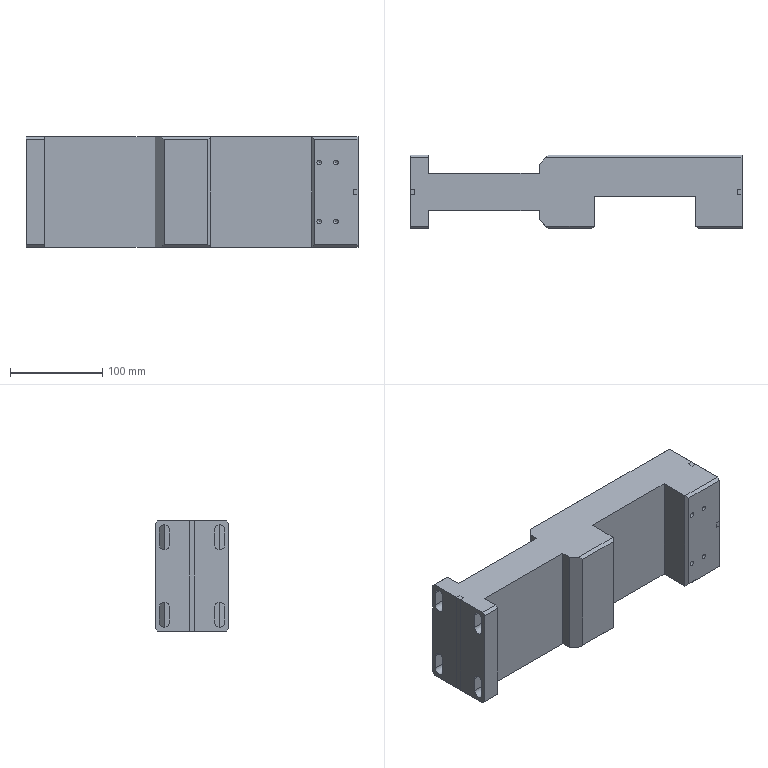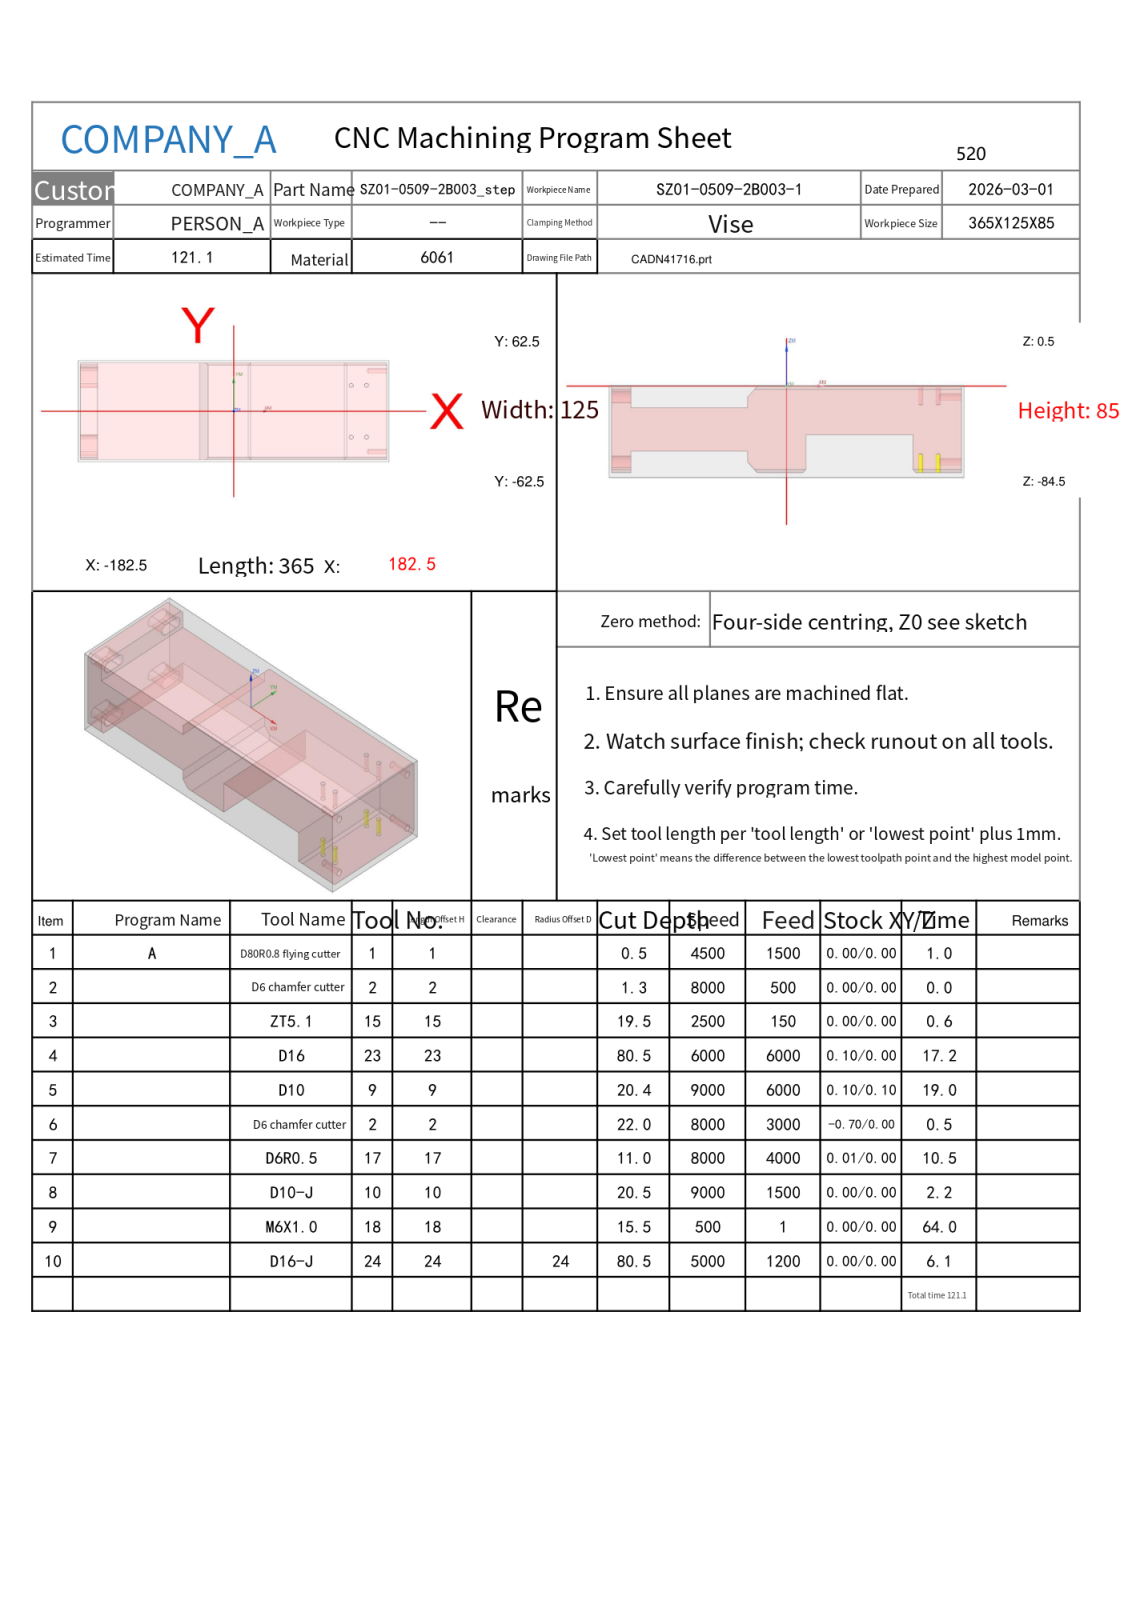NC program | NX | posted by the shop | part box 360 x 80 x 120 mm
Lines 4546 to 6444 of 6444:
N7 T17 M06
(D6R0.5  D=6. R=0.5 H=17 ce=0.01 di=0.00)
G00 G90 G54 X-32.786 Y-63.359 M03 S8000
G43 H17 Z10.788
M08
Z.429
G01 Z-.071 F4000.
Y-58.232
Y58.232
X-32.857 Y58.303 Z-.141
Y-58.303
X-32.927 Y-58.375 Z-.212
X-32.929 Y-58.275
Y58.275
X-32.927 Y58.375
X-32.996 Y58.446 Z-.283
X-33. Y58.275
Y-58.275
X-32.996 Y-58.446
X-33.068 Y-58.517 Z-.354
X-33.071 Y-58.275
Y58.275
X-33.068 Y58.517
X-33.14 Y58.588 Z-.424
X-33.141 Y57.278
Y-57.278
X-33.14 Y-58.588
X-33.21 Y-58.66 Z-.495
X-33.212 Y-58.622
Y58.622
X-33.21 Y58.66
X-33.28 Y58.731 Z-.566
X-33.283 Y58.622
Y-58.622
X-33.28 Y-58.731
X-33.35 Y-58.802 Z-.636
X-33.354 Y-58.622
Y58.622
X-33.35 Y58.802
X-33.421 Y58.873 Z-.707
X-33.424 Y58.622
Y-58.622
X-33.421 Y-58.873
X-33.494 Y-58.944 Z-.778
X-33.495 Y-57.631
Y57.631
X-33.494 Y58.944
X-33.563 Y59.015 Z-.849
X-33.566 Y58.969
Y-58.969
X-33.563 Y-59.015
X-33.633 Y-59.085 Z-.919
X-33.636 Y-58.969
Y58.969
X-33.633 Y59.085
X-33.704 Y59.156 Z-.99
X-33.707 Y58.969
Y-58.969
X-33.704 Y-59.156
X-33.775 Y-59.227 Z-1.061
X-33.778 Y-58.969
Y58.969
X-33.775 Y59.227
X-33.848 Y59.297 Z-1.131
Y57.985
Y-57.985
Y-59.297
X-33.917 Y-59.368 Z-1.202
X-33.919 Y-59.316
Y59.316
X-33.917 Y59.368
X-33.987 Y59.438 Z-1.273
X-33.99 Y59.316
Y-59.316
X-33.987 Y-59.439
X-34.057 Y-59.509 Z-1.344
X-34.061 Y-59.316
Y59.316
X-34.057 Y59.509
X-34.129 Y59.58 Z-1.414
X-34.131 Y58.268
Y-58.268
X-34.129 Y-59.58
X-34.202 Y-59.65 Z-1.485
Y-58.339
Y58.339
Y59.65
X-34.27 Y59.721 Z-1.556
X-34.273 Y59.663
Y-59.663
X-34.27 Y-59.721
X-34.34 Y-59.791 Z-1.626
X-34.343 Y-59.663
Y59.663
X-34.34 Y59.792
X-34.411 Y59.862 Z-1.697
X-34.414 Y59.663
Y-59.663
X-34.411 Y-59.862
X-34.482 Y-59.932 Z-1.768
X-34.485 Y-58.621
Y58.621
X-34.482 Y59.932
X-34.555 Y60.002 Z-1.838
X-34.556 Y58.692
Y-58.692
X-34.555 Y-60.002
X-34.624 Y-60.072 Z-1.909
X-34.626 Y-60.009
Y60.009
X-34.624 Y60.072
X-34.694 Y60.142 Z-1.98
X-34.697 Y60.009
Y-60.009
X-34.694 Y-60.142
X-34.764 Y-60.212 Z-2.051
X-34.768 Y-60.009
Y60.009
X-34.764 Y60.212
X-34.836 Y60.282 Z-2.121
X-34.838 Y58.975
Y-58.975
X-34.836 Y-60.282
X-34.909 Y-60.352 Z-2.192
Y-59.046
Y59.046
Y60.352
X-34.977 Y60.422 Z-2.263
X-34.98 Y60.356
Y-60.356
X-34.977 Y-60.422
X-35.047 Y-60.492 Z-2.333
X-35.051 Y-60.356
Y60.356
X-35.047 Y60.492
X-35.118 Y60.562 Z-2.404
X-35.121 Y60.356
Y-60.356
X-35.118 Y-60.562
X-35.19 Y-60.632 Z-2.475
X-35.192 Y-59.328
Y59.328
X-35.19 Y60.632
X-35.263 Y60.703 Z-2.546
Y59.399
Y-59.399
Y-60.703
X-35.331 Y-60.772 Z-2.616
X-35.333 Y-60.703
Y60.703
X-35.331 Y60.772
X-35.401 Y60.842 Z-2.687
X-35.404 Y60.703
Y-60.703
X-35.401 Y-60.842
X-35.471 Y-60.912 Z-2.758
X-35.475 Y-60.703
Y60.703
X-35.471 Y60.912
X-35.543 Y60.982 Z-2.828
X-35.546 Y59.682
Y-59.682
X-35.543 Y-60.982
X-35.616 Y-61.05 Z-2.899
Y-59.753
Y59.753
Y61.05
X-35.652 Y61.056 Z-2.934
X-35.686 Y61.061 Z-2.97
X-35.687 Y59.823
Y-59.823
X-35.686 Y-61.061
X-35.722 Y-61.062 Z-3.005
X-35.757 Z-3.041
X-35.758 Y-59.894
Y59.894
X-35.757 Y61.062
X-35.793 Y61.063 Z-3.076
X-35.828 Z-3.111
Y59.965
Y-59.965
Y-61.063
X-35.864 Z-3.147
X-35.898 Y-61.064 Z-3.182
X-35.899 Y-60.
Y60.
X-35.898 Y61.064
X-35.934 Z-3.217
X-35.969 Y61.065 Z-3.253
X-35.97 Y60.
Y-60.
X-35.969 Y-61.065
X-36.005 Z-3.288
X-36.04 Z-3.323
X-36.041 Y-60.
Y60.
X-36.04 Y61.065
X-36.076 Y61.066 Z-3.359
X-36.11 Z-3.394
X-36.111 Y60.
Y-60.
X-36.11 Y-61.066
X-36.147 Z-3.429
X-36.181 Y-61.067 Z-3.465
X-36.182 Y-60.
Y60.
X-36.181 Y61.067
X-36.217 Z-3.5
X-36.252 Y61.068 Z-3.536
X-36.253 Y60.
Y-60.
X-36.252 Y-61.067
X-36.288 Y-61.068 Z-3.571
X-36.322 Z-3.606
X-36.323 Y-60.
Y60.
X-36.322 Y61.068
X-36.359 Y61.069 Z-3.642
X-36.393 Z-3.677
X-36.394 Y60.
Y-60.
X-36.393 Y-61.069
X-36.429 Z-3.712
X-36.464 Y-61.07 Z-3.748
X-36.465 Y-60.
Y60.
X-36.464 Y61.07
X-36.5 Z-3.783
X-36.534 Z-3.818
X-36.535 Y60.
Y-60.
X-36.534 Y-61.07
X-36.571 Y-61.071 Z-3.854
X-36.605 Z-3.889
X-36.606 Y-60.
Y60.
X-36.605 Y61.071
X-36.642 Y61.072 Z-3.924
X-36.676 Z-3.96
X-36.677 Y60.
Y-60.
X-36.676 Y-61.072
X-36.712 Z-3.995
X-36.746 Y-61.073 Z-4.031
X-36.748 Y-60.
Y60.
X-36.746 Y61.073
X-36.783 Z-4.066
X-36.817 Z-4.101
X-36.818 Y60.
Y-60.
X-36.817 Y-61.073
X-36.854 Y-61.074 Z-4.137
X-36.888 Z-4.172
X-36.889 Y-60.
Y60.
X-36.888 Y61.074
X-36.924 Y61.075 Z-4.207
X-36.958 Z-4.243
X-36.96 Y61.05
Y-61.05
X-36.958 Y-61.075
X-36.995 Z-4.278
X-37.029 Y-61.076 Z-4.313
X-37.03 Y-61.05
Y61.05
X-37.029 Y61.076
X-37.066 Z-4.349
X-37.1 Z-4.384
X-37.101 Y61.05
Y-61.05
X-37.1 Y-61.076
X-37.137 Y-61.077 Z-4.419
X-37.17 Z-4.455
X-37.172 Y-61.05
Y61.05
X-37.17 Y61.077
X-37.207 Z-4.49
X-37.241 Y61.078 Z-4.525
X-37.243 Y61.05
Y-61.05
X-37.241 Y-61.078
X-37.278 Z-4.561
X-37.312 Z-4.596
X-37.313 Y-61.05
Y61.05
X-37.312 Y61.078
X-37.349 Y61.079 Z-4.632
X-37.383 Z-4.667
X-37.384 Y61.05
Y-61.05
X-37.383 Y-61.079
X-37.419 Z-4.702
X-37.453 Z-4.738
X-37.455 Y-61.05
Y61.05
X-37.453 Y61.079
X-37.49 Y61.08 Z-4.773
X-37.524 Z-4.808
X-37.525 Y61.05
Y-61.05
X-37.524 Y-61.08
X-37.561 Z-4.844
X-37.595 Z-4.879
X-37.596 Y-61.05
Y61.05
X-37.595 Y61.08
X-37.632 Y61.081 Z-4.914
X-37.665 Z-4.95
X-37.667 Y61.05
Y-61.05
X-37.665 Y-61.081
X-37.702 Z-4.985
X-37.736 Z-5.02
X-37.738 Y-61.05
Y61.05
X-37.736 Y61.081
X-37.773 Y61.082 Z-5.056
X-37.807 Z-5.091
X-37.808 Y61.05
Y-61.05
X-37.807 Y-61.082
X-37.844 Z-5.127
X-37.877 Z-5.162
X-37.879 Y-61.05
Y61.05
X-37.877 Y61.082
X-37.914 Y61.083 Z-5.197
X-37.948 Z-5.233
X-37.95 Y61.05
Y-61.05
X-37.948 Y-61.083
X-37.985 Z-5.268
X-38.019 Z-5.303
X-38.02 Y-61.05
Y61.05
X-38.019 Y61.083
X-38.056 Y61.084 Z-5.339
X-38.089 Z-5.374
X-38.091 Y61.05
Y-61.05
X-38.089 Y-61.084
X-38.126 Z-5.409
X-38.16 Z-5.445
X-38.162 Y-61.05
Y61.05
X-38.16 Y61.084
X-38.197 Z-5.48
X-38.231 Y61.085 Z-5.515
X-38.233 Y61.05
Y-61.05
X-38.231 Y-61.085
X-38.268 Z-5.551
X-38.302 Z-5.586
X-38.303 Y-61.05
Y61.05
X-38.302 Y61.085
X-38.339 Z-5.622
X-38.372 Y61.086 Z-5.657
X-38.374 Y61.05
Y-61.05
X-38.372 Y-61.086
X-38.409 Z-5.692
X-38.443 Z-5.728
X-38.445 Y-61.05
Y61.05
X-38.443 Y61.086
X-38.48 Z-5.763
X-38.514 Y61.087 Z-5.798
X-38.515 Y61.05
Y-61.05
X-38.514 Y-61.087
X-38.551 Z-5.834
X-38.584 Z-5.869
X-38.586 Y-61.05
Y61.05
X-38.584 Y61.087
X-38.621 Z-5.904
X-38.655 Z-5.94
X-38.657 Y61.05
Y-61.05
X-38.655 Y-61.087
X-38.692 Z-5.975
X-38.726 Z-6.01
X-38.728 Y-60.
Y61.05
X-38.726 Y61.088
X-38.763 Z-6.046
X-38.796 Z-6.081
X-38.798 Y61.05
Y-61.05
X-38.796 Y-61.088
X-38.834 Z-6.116
X-38.867 Z-6.152
X-38.869 Y-61.05
Y61.05
X-38.867 Y61.088
X-38.904 Z-6.187
X-38.938 Z-6.223
X-38.94 Y61.05
Y-61.05
X-38.938 Y-61.088
X-38.975 Z-6.258
X-39.009 Z-6.293
X-39.01 Y-61.05
Y61.05
X-39.009 Y61.088
X-39.046 Z-6.329
X-39.079 Z-6.364
X-39.081 Y61.05
Y-61.05
X-39.079 Y-61.088
X-39.116 Z-6.399
X-39.152 Z-6.435
Y-60.
Y60.
Y61.088
X-39.187 Z-6.47
X-39.221 Z-6.505
X-39.222 Y61.05
Y-61.05
X-39.221 Y-61.088
X-39.258 Z-6.541
X-39.291 Y-61.089 Z-6.576
X-39.293 Y-61.05
Y61.05
X-39.291 Y61.088
X-39.329 Z-6.611
X-39.362 Y61.089 Z-6.647
X-39.364 Y61.05
Y-61.05
X-39.362 Y-61.089
X-39.399 Z-6.682
X-39.433 Z-6.718
X-39.435 Y-61.05
Y61.05
X-39.433 Y61.089
X-39.47 Z-6.753
X-39.504 Z-6.788
X-39.505 Y61.05
Y-61.05
X-39.504 Y-61.089
X-39.541 Z-6.824
X-39.574 Z-6.859
X-39.576 Y-61.05
Y61.05
X-39.574 Y61.089
X-39.611 Z-6.894
X-39.645 Z-6.93
X-39.647 Y61.05
Y-61.05
X-39.645 Y-61.089
X-39.682 Z-6.965
X-39.716 Z-7.
X-39.717 Y-61.05
Y61.05
X-39.716 Y61.089
X-39.753 Z-7.036
X-39.786 Z-7.071
X-39.788 Y61.05
Y-61.05
X-39.786 Y-61.089
X-39.824 Z-7.106
X-39.857 Z-7.142
X-39.859 Y-61.05
Y61.05
X-39.857 Y61.089
X-39.894 Z-7.177
X-39.928 Z-7.212
X-39.93 Y61.05
Y-61.05
X-39.928 Y-61.089
X-39.965 Z-7.248
X-39.998 Z-7.283
X-40. Y-61.05
Y61.05
X-39.998 Y61.089
X-40.036 Z-7.319
X-40.069 Z-7.354
X-40.071 Y61.05
Y-61.05
X-40.069 Y-61.089
X-40.106 Z-7.389
X-40.14 Z-7.425
X-40.142 Y-61.05
Y61.05
X-40.14 Y61.089
X-40.177 Z-7.46
X-40.211 Z-7.495
X-40.212 Y61.05
Y-61.05
X-40.211 Y-61.089
X-40.248 Z-7.531
X-40.281 Z-7.566
X-40.283 Y-61.05
Y61.05
X-40.281 Y61.089
X-40.319 Z-7.601
X-40.352 Y61.088 Z-7.637
X-40.354 Y61.05
Y-61.05
X-40.352 Y-61.088
X-40.389 Z-7.672
X-40.423 Z-7.707
X-40.425 Y-61.05
Y61.05
X-40.423 Y61.088
X-40.46 Z-7.743
X-40.493 Z-7.778
X-40.495 Y61.05
Y-61.05
X-40.493 Y-61.088
X-40.531 Z-7.814
X-40.564 Z-7.849
X-40.566 Y-61.05
Y61.05
X-40.564 Y61.088
X-40.601 Z-7.884
X-40.635 Y61.087 Z-7.92
X-40.637 Y61.05
Y-61.05
X-40.635 Y-61.087
X-40.672 Z-7.955
X-40.706 Z-7.99
X-40.707 Y-61.05
Y61.05
X-40.706 Y61.087
X-40.743 Z-8.026
X-40.776 Z-8.061
X-40.778 Y61.05
Y-61.05
X-40.776 Y-61.087
X-40.813 Z-8.096
X-40.847 Y-61.086 Z-8.132
X-40.849 Y-61.05
Y61.05
X-40.847 Y61.087
X-40.884 Z-8.167
X-40.918 Y61.086 Z-8.202
X-40.92 Y61.05
Y-61.05
X-40.918 Y-61.086
X-40.955 Z-8.238
X-40.989 Z-8.273
X-40.99 Y-61.05
Y61.05
X-40.989 Y61.086
X-41.026 Z-8.309
X-41.059 Z-8.344
X-41.061 Y61.05
Y-61.05
X-41.059 Y-61.086
X-41.096 Z-8.379
X-41.13 Z-8.415
X-41.132 Y-61.05
Y61.05
X-41.13 Y61.086
X-41.167 Y61.085 Z-8.45
X-41.201 Z-8.485
X-41.202 Y61.05
Y-61.05
X-41.201 Y-61.085
X-41.238 Z-8.521
X-41.271 Z-8.556
X-41.273 Y-61.05
Y61.05
X-41.271 Y61.085
X-41.308 Z-8.591
X-41.342 Z-8.627
X-41.344 Y61.05
Y-61.05
X-41.342 Y-61.085
X-41.379 Z-8.662
X-41.413 Y-61.084 Z-8.697
X-41.415 Y-61.05
Y61.05
X-41.413 Y61.084
X-41.45 Z-8.733
X-41.484 Z-8.768
X-41.485 Y61.05
Y-61.05
X-41.484 Y-61.084
X-41.521 Z-8.803
X-41.554 Z-8.839
X-41.556 Y-61.05
Y61.05
X-41.554 Y61.084
X-41.591 Y61.083 Z-8.874
X-41.625 Z-8.91
X-41.627 Y61.05
Y-61.05
X-41.625 Y-61.083
X-41.662 Z-8.945
X-41.696 Z-8.98
X-41.697 Y-61.05
Y61.05
X-41.696 Y61.083
X-41.733 Y61.082 Z-9.016
X-41.766 Z-9.051
X-41.768 Y61.05
Y-61.05
X-41.766 Y-61.082
X-41.803 Z-9.086
X-41.837 Z-9.122
X-41.839 Y-61.05
Y61.05
X-41.837 Y61.082
X-41.874 Z-9.157
X-41.908 Y61.081 Z-9.192
X-41.909 Y61.05
Y-61.05
X-41.908 Y-61.081
X-41.945 Z-9.228
X-41.979 Z-9.263
X-41.98 Y-61.05
Y61.05
X-41.979 Y61.081
X-42.016 Z-9.298
X-42.049 Y61.08 Z-9.334
X-42.051 Y61.05
Y-61.05
X-42.049 Y-61.08
X-42.086 Z-9.369
X-42.12 Z-9.405
X-42.122 Y-61.05
Y61.05
X-42.12 Y61.08
X-42.157 Z-9.44
X-42.191 Y61.079 Z-9.475
X-42.192 Y61.05
Y-61.05
X-42.191 Y-61.079
X-42.228 Z-9.511
X-42.262 Z-9.546
X-42.263 Y-61.05
Y61.05
X-42.262 Y61.079
X-42.298 Z-9.581
X-42.332 Y61.078 Z-9.617
X-42.334 Y61.05
Y-61.05
X-42.332 Y-61.078
X-42.369 Z-9.652
X-42.403 Z-9.687
X-42.404 Y-61.05
Y61.05
X-42.403 Y61.078
X-42.44 Z-9.723
X-42.474 Z-9.758
X-42.475 Y61.05
Y-61.05
X-42.474 Y-61.077
X-42.511 Z-9.793
X-42.545 Z-9.829
X-42.546 Y-61.05
Y61.05
X-42.544 Y61.077
X-42.581 Z-9.864
X-42.616 Z-9.899
X-42.617 Y60.
Y-60.
X-42.616 Y-61.077
X-42.652 Y-61.076 Z-9.935
X-42.686 Z-9.97
X-42.687 Y-61.05
Y61.05
X-42.686 Y61.076
X-42.723 Z-10.006
X-42.757 Z-10.041
X-42.758 Y61.05
Y-61.05
X-42.757 Y-61.076
X-42.793 Y-61.075 Z-10.076
X-42.827 Z-10.112
X-42.829 Y-61.05
Y61.05
X-42.827 Y61.075
X-42.864 Z-10.147
X-42.898 Z-10.182
Y-61.075
X-42.935 Y-61.074 Z-10.218
X-42.969 Z-10.253
Y61.074
X-43.001 Z-10.284
X-43.031 Z-10.315
Y-61.074
X-43.063 Z-10.346
X-43.092 Y-61.073 Z-10.377
Y61.073
X-43.125 Z-10.407
X-43.154 Z-10.438
Y-61.073
X-43.186 Z-10.469
X-43.216 Z-10.5
Y61.073
G00 Z10.788
G00 G90 X-153.773 Y-59.784 M03 S8000
Z10.788
Z.429
G01 Z-.071 F4000.
X-158.926 Y-59.785
X-181.074 Y-59.788
Y-59.823 Z-.106
Y-59.858 Z-.141
X-158.926 Y-59.856
Y-59.894 Z-.177
Y-59.926 Z-.212
X-159.074 Y-59.929
X-180.
X-181.074
X-181.075 Y-59.965 Z-.247
Y-60. Z-.283
X-180.
X-159.074
X-158.925 Y-59.997
Y-60.035 Z-.318
Y-60.068 Z-.354
X-159.074 Y-60.071
X-180.
X-181.075
Y-60.106 Z-.389
X-181.076 Y-60.141 Z-.424
X-180.
X-159.074
X-158.925 Y-60.138
X-158.924 Y-60.177 Z-.46
Y-60.209 Z-.495
X-159.074 Y-60.212
X-180.
X-181.076
Y-60.247 Z-.53
Y-60.283 Z-.566
X-180.
X-159.074
X-158.924 Y-60.28
Y-60.318 Z-.601
X-158.923 Y-60.351 Z-.636
X-159.074 Y-60.354
X-180.
X-181.077 Y-60.353
Y-60.389 Z-.672
Y-60.424 Z-.707
X-180.
X-159.074
X-158.923 Y-60.421
Y-60.46 Z-.742
Y-60.492 Z-.778
X-159.074 Y-60.495
X-180.
X-181.077
X-181.078 Y-60.53 Z-.813
Y-60.566 Z-.849
X-180.
X-159.074
X-158.922 Y-60.563
Y-60.601 Z-.884
Y-60.634 Z-.919
X-159.074 Y-60.636
X-180.
X-181.078
Y-60.672 Z-.955
Y-60.707 Z-.99
X-180.
X-159.074
X-158.922 Y-60.704
X-158.921 Y-60.742 Z-1.025
Y-60.775 Z-1.061
X-159.074 Y-60.778
X-180.
X-181.079
Y-60.813 Z-1.096
Y-60.848 Z-1.131
X-180.
X-159.074
X-158.921 Y-60.846
Y-60.884 Z-1.167
Y-60.916 Z-1.202
X-159.074 Y-60.919
X-180.
X-181.079
Y-60.955 Z-1.237
Y-60.99 Z-1.273
X-180.
X-159.074
X-158.921 Y-60.987
Y-61.025 Z-1.308
Y-61.058 Z-1.344
X-159.074 Y-61.061
X-180.
X-181.079
Y-61.096 Z-1.379
Y-61.131 Z-1.414
X-180.
X-160.
X-158.921
Y-61.167 Z-1.45
Y-61.199 Z-1.485
X-159.074 Y-61.202
X-180.
X-181.079
Y-61.237 Z-1.52
Y-61.273 Z-1.556
X-180.
X-159.074
X-158.921 Y-61.27
Y-61.308 Z-1.591
Y-61.341 Z-1.626
X-159.074 Y-61.343
X-180.
X-181.079
Y-61.379 Z-1.662
Y-61.414 Z-1.697
X-180.
X-159.074
X-158.921 Y-61.411
Y-61.45 Z-1.732
Y-61.482 Z-1.768
X-159.074 Y-61.485
X-180.
X-181.079
Y-61.52 Z-1.803
Y-61.556 Z-1.838
X-180.
X-159.074
X-158.921 Y-61.553
Y-61.591 Z-1.874
Y-61.623 Z-1.909
X-159.074 Y-61.626
X-180.
X-181.079
Y-61.662 Z-1.945
Y-61.697 Z-1.98
X-180.
X-159.074
X-158.921 Y-61.694
Y-61.732 Z-2.015
Y-61.765 Z-2.051
X-159.074 Y-61.768
X-180.
X-181.079
Y-61.803 Z-2.086
Y-61.838 Z-2.121
X-180.
X-159.074
X-158.921 Y-61.836
Y-61.874 Z-2.157
Y-61.906 Z-2.192
X-159.074 Y-61.909
X-180.
X-181.079
Y-61.944 Z-2.227
Y-61.98 Z-2.263
X-180.
X-159.074
X-158.922 Y-61.977
Y-62.015 Z-2.298
Y-62.048 Z-2.333
X-159.074 Y-62.051
X-180.
X-181.078
Y-62.086 Z-2.369
Y-62.121 Z-2.404
X-180.
X-159.074
X-158.922 Y-62.118
Y-62.157 Z-2.44
Y-62.189 Z-2.475
X-159.074 Y-62.192
X-180.
X-181.078
X-181.077 Y-62.227 Z-2.51
Y-62.263 Z-2.546
X-180.
X-159.074
X-158.923 Y-62.26
Y-62.298 Z-2.581
Y-62.331 Z-2.616
X-159.074 Y-62.333
X-180.
X-181.077
Y-62.369 Z-2.652
X-181.076 Y-62.404 Z-2.687
X-180.
X-159.074
X-158.924 Y-62.401
Y-62.439 Z-2.722
Y-62.472 Z-2.758
X-159.074 Y-62.475
X-180.
X-181.076
Y-62.51 Z-2.793
Y-62.546 Z-2.828
X-180.
X-159.074
X-158.924 Y-62.543
X-158.925 Y-62.581 Z-2.864
Y-62.613 Z-2.899
X-159.074 Y-62.616
X-180.
X-181.075
Y-62.652 Z-2.934
Y-62.687 Z-2.97
X-180.
X-159.074
X-158.925 Y-62.684
Y-62.722 Z-3.005
Y-62.755 Z-3.041
X-159.074 Y-62.758
X-180.
X-181.075
X-181.074 Y-62.793 Z-3.076
Y-62.828 Z-3.111
X-180.
X-159.074
X-158.926 Y-62.825
Y-62.864 Z-3.147
Y-62.896 Z-3.182
X-181.074 Y-62.899
Y-62.934 Z-3.217
X-181.073 Y-62.97 Z-3.253
X-158.927 Y-62.967
Y-63.001 Z-3.284
Y-63.029 Z-3.315
X-181.073 Y-63.032
Y-63.063 Z-3.345
Y-63.093 Z-3.376
X-158.927 Y-63.091
Y-63.124 Z-3.407
X-158.928 Y-63.152 Z-3.438
X-181.073 Y-63.155
X-181.072 Y-63.186 Z-3.469
Y-63.217 Z-3.5
X-158.928 Y-63.214
G00 Z10.788
X-186.221 Y59.788
Z.429
G01 Z-.071
X-181.074
X-158.926 Y59.785
Y59.823 Z-.106
Y59.856 Z-.141
X-181.074 Y59.858
Y59.894 Z-.177
Y59.929 Z-.212
X-180.
X-159.074
X-158.926 Y59.926
X-158.925 Y59.965 Z-.247
Y59.997 Z-.283
X-159.074 Y60.
X-180.
X-181.075
Y60.035 Z-.318
Y60.071 Z-.354
X-180.
X-159.074
X-158.925 Y60.068
Y60.106 Z-.389
Y60.138 Z-.424
X-159.074 Y60.141
X-180.
X-181.076
Y60.177 Z-.46
Y60.212 Z-.495
X-180.
X-159.074
X-158.924 Y60.209
Y60.247 Z-.53
Y60.28 Z-.566
X-159.074 Y60.283
X-180.
X-181.076
Y60.318 Z-.601
X-181.077 Y60.353 Z-.636
X-180. Y60.354
X-159.074
X-158.923 Y60.351
Y60.389 Z-.672
Y60.421 Z-.707
X-159.074 Y60.424
X-180.
X-181.077
Y60.46 Z-.742
Y60.495 Z-.778
X-180.
X-159.074
X-158.923 Y60.492
X-158.922 Y60.53 Z-.813
Y60.563 Z-.849
X-159.074 Y60.566
X-180.
X-181.078
Y60.601 Z-.884
Y60.636 Z-.919
X-180.
X-159.074
X-158.922 Y60.634
Y60.672 Z-.955
Y60.704 Z-.99
X-159.074 Y60.707
X-180.
X-181.078
X-181.079 Y60.742 Z-1.025
Y60.778 Z-1.061
X-180.
X-159.074
X-158.921 Y60.775
Y60.813 Z-1.096
Y60.846 Z-1.131
X-159.074 Y60.848
X-180.
X-181.079
Y60.884 Z-1.167
Y60.919 Z-1.202
X-180.
X-159.074
X-158.921 Y60.916
Y60.955 Z-1.237
Y60.987 Z-1.273
X-159.074 Y60.99
X-180.
X-181.079
Y61.025 Z-1.308
Y61.061 Z-1.344
X-180.
X-159.074
X-158.921 Y61.058
Y61.096 Z-1.379
Y61.131 Z-1.414
X-160.
X-180.
X-181.079
Y61.167 Z-1.45
Y61.202 Z-1.485
X-180.
X-159.074
X-158.921 Y61.199
Y61.237 Z-1.52
Y61.27 Z-1.556
X-159.074 Y61.273
X-180.
X-181.079
Y61.308 Z-1.591
Y61.343 Z-1.626
X-180.
X-159.074
X-158.921 Y61.341
Y61.379 Z-1.662
Y61.411 Z-1.697
X-159.074 Y61.414
X-180.
X-181.079
Y61.45 Z-1.732
Y61.485 Z-1.768
X-180.
X-159.074
X-158.921 Y61.482
Y61.52 Z-1.803
Y61.553 Z-1.838
X-159.074 Y61.556
X-180.
X-181.079
Y61.591 Z-1.874
Y61.626 Z-1.909
X-180.
X-159.074
X-158.921 Y61.623
Y61.662 Z-1.945
Y61.694 Z-1.98
X-159.074 Y61.697
X-180.
X-181.079
Y61.732 Z-2.015
Y61.768 Z-2.051
X-180.
X-159.074
X-158.921 Y61.765
Y61.803 Z-2.086
Y61.836 Z-2.121
X-159.074 Y61.838
X-180.
X-181.079
Y61.874 Z-2.157
Y61.909 Z-2.192
X-180.
X-159.074
X-158.921 Y61.906
Y61.944 Z-2.227
X-158.922 Y61.977 Z-2.263
X-159.074 Y61.98
X-180.
X-181.079
X-181.078 Y62.015 Z-2.298
Y62.051 Z-2.333
X-180.
X-159.074
X-158.922 Y62.048
Y62.086 Z-2.369
Y62.118 Z-2.404
X-159.074 Y62.121
X-180.
X-181.078
Y62.157 Z-2.44
Y62.192 Z-2.475
X-180.
X-159.074
X-158.922 Y62.189
X-158.923 Y62.227 Z-2.51
Y62.26 Z-2.546
X-159.074 Y62.263
X-180.
X-181.077
Y62.298 Z-2.581
Y62.333 Z-2.616
X-180.
X-159.074
X-158.923 Y62.331
Y62.369 Z-2.652
X-158.924 Y62.401 Z-2.687
X-159.074 Y62.404
X-180.
X-181.076
Y62.439 Z-2.722
Y62.475 Z-2.758
X-180.
X-159.074
X-158.924 Y62.472
Y62.51 Z-2.793
Y62.543 Z-2.828
X-159.074 Y62.546
X-180.
X-181.076
X-181.075 Y62.581 Z-2.864
Y62.616 Z-2.899
X-180.
X-159.074
X-158.925 Y62.613
Y62.652 Z-2.934
Y62.684 Z-2.97
X-159.074 Y62.687
X-180.
X-181.075
Y62.722 Z-3.005
Y62.758 Z-3.041
X-180.
X-159.074
X-158.925 Y62.755
X-158.926 Y62.793 Z-3.076
Y62.825 Z-3.111
X-159.074 Y62.828
X-180.
X-181.074
Y62.864 Z-3.147
Y62.899 Z-3.182
X-158.926 Y62.896
Y62.934 Z-3.217
X-158.927 Y62.967 Z-3.253
X-181.073 Y62.97
Y63.001 Z-3.284
Y63.032 Z-3.315
X-158.927 Y63.029
Y63.063 Z-3.345
Y63.091 Z-3.376
X-181.073 Y63.093
Y63.124 Z-3.407
Y63.155 Z-3.438
X-158.928 Y63.152
Y63.186 Z-3.469
Y63.214 Z-3.5
X-181.072 Y63.217
G00 Z10.788
X-36.361 Y59.785
Z.429
G01 Z-.071
X-31.233
X181.074 Y59.787
Y59.823 Z-.106
Y59.857 Z-.141
X-31.304 Y59.855
X-31.376 Y59.927 Z-.212
X-30.066 Y59.929
X180.
X181.074 Y59.928
X181.075 Y59.965 Z-.247
Y59.999 Z-.283
X180. Y60.
X-30.136
X-31.447
X-31.518 Y60.068 Z-.354
X-31.447 Y60.071
X180.
X181.075 Y60.069
Y60.106 Z-.389
Y60.14 Z-.424
X180. Y60.141
X-31.447
X-31.59 Y60.138
X-31.661 Y60.209 Z-.495
X-31.447 Y60.212
X180.
X181.076 Y60.211
Y60.247 Z-.53
Y60.282 Z-.566
X180. Y60.283
X-30.419
X-31.733 Y60.281
X-31.804 Y60.353 Z-.636
X-30.49 Y60.354
X180.
X181.076 Y60.352
X181.077 Y60.389 Z-.672
Y60.423 Z-.707
X180. Y60.424
X-31.793
X-31.875 Y60.421
X-31.946 Y60.492 Z-.778
X-31.793 Y60.495
X180.
X181.077 Y60.494
Y60.53 Z-.813
X181.078 Y60.564 Z-.849
X180. Y60.566
X-31.793
X-32.017 Y60.563
X-32.088 Y60.635 Z-.919
X-30.773 Y60.636
X181.053
X181.078 Y60.635
Y60.672 Z-.955
Y60.706 Z-.99
X181.053 Y60.707
X-30.844
X-32.158 Y60.706
X-32.229 Y60.775 Z-1.061
X-32.14 Y60.778
X181.053
X181.079 Y60.776
Y60.813 Z-1.096
Y60.847 Z-1.131
X181.053 Y60.848
X-32.14
X-32.3 Y60.845
X-32.371 Y60.916 Z-1.202
X-32.14 Y60.919
X181.053
X181.079 Y60.918
Y60.955 Z-1.237
Y60.989 Z-1.273
X181.053 Y60.99
X-31.126
X-32.442 Y60.988
X-32.512 Y61.059 Z-1.344
X-32.487 Y61.061
X181.053
X181.079 Y61.059
Y61.096 Z-1.379
Y61.131 Z-1.414
X180.
X-31.268
X-32.583
X-32.654 Y61.199 Z-1.485
X-32.487 Y61.202
X181.053
X181.079 Y61.201
Y61.237 Z-1.52
Y61.271 Z-1.556
X181.053 Y61.273
X-32.487
X-32.725 Y61.27
X-32.796 Y61.342 Z-1.626
X-31.48 Y61.343
X181.053
X181.079 Y61.342
Y61.379 Z-1.662
Y61.413 Z-1.697
X181.053 Y61.414
X-32.833
X-32.866 Y61.412
X-32.937 Y61.482 Z-1.768
X-32.833 Y61.485
X181.053
X181.079 Y61.484
Y61.52 Z-1.803
Y61.554 Z-1.838
X181.053 Y61.556
X-32.833
X-33.007 Y61.552
X-33.077 Y61.623 Z-1.909
X-32.833 Y61.626
X181.053
X181.079 Y61.625
Y61.662 Z-1.945
Y61.696 Z-1.98
X181.053 Y61.697
X-31.833
X-33.147 Y61.696
X-33.217 Y61.766 Z-2.051
X-33.18 Y61.768
X181.053
X181.079 Y61.766
Y61.803 Z-2.086
Y61.837 Z-2.121
X181.053 Y61.838
X-33.18
X-33.288 Y61.835
X-33.358 Y61.906 Z-2.192
X-33.18 Y61.909
X181.053
X181.079 Y61.908
Y61.944 Z-2.227
X181.078 Y61.979 Z-2.263
X181.053 Y61.98
X-33.18
X-33.428 Y61.977
X-33.498 Y62.049 Z-2.333
X-32.187 Y62.051
X181.053
X181.078 Y62.049
Y62.086 Z-2.369
Y62.12 Z-2.404
X181.053 Y62.121
X-33.527
X-33.569 Y62.119
X-33.639 Y62.189 Z-2.475
X-33.527 Y62.192
X180.
X181.077 Y62.191
Y62.227 Z-2.51
Y62.261 Z-2.546
X180. Y62.263
X-33.527
X-33.709 Y62.259
X-33.779 Y62.33 Z-2.616
X-33.527 Y62.333
X180.
X181.077 Y62.332
Y62.369 Z-2.652
X181.076 Y62.403 Z-2.687
X180. Y62.404
X-32.541
X-33.85 Y62.403
X-33.92 Y62.473 Z-2.758
X-33.873 Y62.475
X180.
X181.076 Y62.474
Y62.51 Z-2.793
Y62.544 Z-2.828
X180. Y62.546
X-33.873
X-33.99 Y62.542
X-34.06 Y62.612 Z-2.899
X-33.873 Y62.616
X180.
X181.075 Y62.615
Y62.652 Z-2.934
Y62.686 Z-2.97
X180. Y62.687
X-33.873
X-34.13 Y62.684
X-34.201 Y62.757 Z-3.041
X-32.894 Y62.758
X180.
X181.075 Y62.757
X181.074 Y62.793 Z-3.076
Y62.827 Z-3.111
X180. Y62.828
X-34.22
X-34.271 Y62.826
X-34.246 Y62.898 Z-3.182
X181.074
Y62.934 Z-3.217
X181.073 Y62.969 Z-3.253
X-34.198
X-34.136 Y63.029 Z-3.315
X181.073 Y63.031
Y63.063 Z-3.345
Y63.092 Z-3.376
X-34.075 Y63.09
X-34.013 Y63.152 Z-3.438
X181.072 Y63.154
Y63.186 Z-3.469
Y63.216 Z-3.5
X-33.951 Y63.214
G00 Z10.788
X186.223 Y-59.787
Z.429
G01 Z-.071
X181.074
X-31.233 Y-59.785
X-31.304 Y-59.855 Z-.141
X181.074 Y-59.857
Y-59.894 Z-.177
Y-59.928 Z-.212
X180. Y-59.929
X-30.066
X-31.376 Y-59.927
X-31.447 Y-60. Z-.283
X-30.136
X180.
X181.075 Y-59.999
Y-60.035 Z-.318
Y-60.069 Z-.354
X180. Y-60.071
X-31.447
X-31.518 Y-60.068
X-31.59 Y-60.138 Z-.424
X-31.447 Y-60.141
X180.
X181.075 Y-60.14
X181.076 Y-60.177 Z-.46
Y-60.211 Z-.495
X180. Y-60.212
X-31.447
X-31.661 Y-60.209
X-31.733 Y-60.281 Z-.566
X-30.419 Y-60.283
X180.
X181.076 Y-60.282
Y-60.318 Z-.601
Y-60.352 Z-.636
X180. Y-60.354
X-30.49
X-31.804 Y-60.353
X-31.875 Y-60.421 Z-.707
X-31.793 Y-60.424
X180.
X181.077 Y-60.423
Y-60.46 Z-.742
Y-60.494 Z-.778
X180. Y-60.495
X-31.793
X-31.946 Y-60.492
X-32.017 Y-60.563 Z-.849
X-31.793 Y-60.566
X180.
X181.078 Y-60.564
Y-60.601 Z-.884
Y-60.635 Z-.919
X181.053 Y-60.636
X-30.773
X-32.088 Y-60.635
X-32.158 Y-60.706 Z-.99
X-30.844 Y-60.707
X181.053
X181.078 Y-60.706
X181.079 Y-60.742 Z-1.025
Y-60.776 Z-1.061
X181.053 Y-60.778
X-32.14
X-32.229 Y-60.775
X-32.3 Y-60.845 Z-1.131
X-32.14 Y-60.848
X181.053
X181.079 Y-60.847
Y-60.884 Z-1.167
Y-60.918 Z-1.202
X181.053 Y-60.919
X-32.14
X-32.371 Y-60.916
X-32.442 Y-60.988 Z-1.273
X-31.126 Y-60.99
X181.053
X181.079 Y-60.989
Y-61.025 Z-1.308
Y-61.059 Z-1.344
X181.053 Y-61.061
X-32.487
X-32.512 Y-61.059
X-32.583 Y-61.131 Z-1.414
X-31.268
X180.94
X181.08 Y-61.13
Y-61.167 Z-1.45
X181.079 Y-61.201 Z-1.485
X181.053 Y-61.202
X-32.487
X-32.654 Y-61.199
X-32.725 Y-61.27 Z-1.556
X-32.487 Y-61.273
X181.053
X181.079 Y-61.271
Y-61.308 Z-1.591
Y-61.342 Z-1.626
X181.053 Y-61.343
X-31.48
X-32.796 Y-61.342
X-32.866 Y-61.412 Z-1.697
X-32.833 Y-61.414
X181.053
X181.079 Y-61.413
Y-61.45 Z-1.732
Y-61.484 Z-1.768
X181.053 Y-61.485
X-32.833
X-32.937 Y-61.482
X-33.007 Y-61.552 Z-1.838
X-32.833 Y-61.556
X181.053
X181.079 Y-61.554
Y-61.591 Z-1.874
Y-61.625 Z-1.909
X181.053 Y-61.626
X-32.833
X-33.077 Y-61.623
X-33.147 Y-61.696 Z-1.98
X-31.833 Y-61.697
X181.053
X181.079 Y-61.696
Y-61.732 Z-2.015
Y-61.766 Z-2.051
X181.053 Y-61.768
X-33.18
X-33.217 Y-61.766
X-33.288 Y-61.835 Z-2.121
X-33.18 Y-61.838
X181.053
X181.079 Y-61.837
Y-61.874 Z-2.157
Y-61.908 Z-2.192
X181.053 Y-61.909
X-33.18
X-33.358 Y-61.906
X-33.428 Y-61.977 Z-2.263
X-33.18 Y-61.98
X181.053
X181.078 Y-61.979
Y-62.015 Z-2.298
Y-62.049 Z-2.333
X181.053 Y-62.051
X-32.187
X-33.498 Y-62.049
X-33.569 Y-62.119 Z-2.404
X-33.527 Y-62.121
X181.053
X181.078 Y-62.12
Y-62.157 Z-2.44
X181.077 Y-62.191 Z-2.475
X180. Y-62.192
X-33.527
X-33.639 Y-62.189
X-33.709 Y-62.259 Z-2.546
X-33.527 Y-62.263
X180.
X181.077 Y-62.261
Y-62.298 Z-2.581
Y-62.332 Z-2.616
X180. Y-62.333
X-33.527
X-33.779 Y-62.33
X-33.85 Y-62.403 Z-2.687
X-32.541 Y-62.404
X180.
X181.076 Y-62.403
Y-62.439 Z-2.722
Y-62.474 Z-2.758
X180. Y-62.475
X-33.873
X-33.92 Y-62.473
X-33.99 Y-62.542 Z-2.828
X-33.873 Y-62.546
X180.
X181.076 Y-62.544
X181.075 Y-62.581 Z-2.864
Y-62.615 Z-2.899
X180. Y-62.616
X-33.873
X-34.06 Y-62.612
X-34.13 Y-62.684 Z-2.97
X-33.873 Y-62.687
X180.
X181.075 Y-62.686
Y-62.722 Z-3.005
Y-62.757 Z-3.041
X180. Y-62.758
X-32.894
X-34.201 Y-62.757
X-34.271 Y-62.826 Z-3.111
X-34.22 Y-62.828
X180.
X181.074 Y-62.827
Y-62.864 Z-3.147
Y-62.898 Z-3.182
X-34.246
X-34.198 Y-62.969 Z-3.253
X181.073
Y-63.001 Z-3.284
Y-63.031 Z-3.315
X-34.136 Y-63.029
X-34.075 Y-63.09 Z-3.376
X181.073 Y-63.092
X181.072 Y-63.124 Z-3.407
Y-63.154 Z-3.438
X-34.013 Y-63.152
X-33.951 Y-63.214 Z-3.5
X181.072 Y-63.216
G00 Z10.788
G91 G28 Z0.0
M05
M09
G91 G28 Z0.0
M01
N8 T10 M06
(D10-J  D=10. R=0. H=10 ce=0.30 di=0.00)
G00 G90 G54 X-100. Y-68. M03 S9000
G43 H10 Z50.
M08
Z-19.5
G01 Z-20. F1500.
Y-61.
X-154.7
Y61.
X-45.3
Y-61.
X-100.
Y-54.
X-147.7
Y54.
X-52.3
Y-54.
X-100.
Y-47.
X-140.7
Y47.
X-59.3
Y-47.
X-100.
Y-40.
X-133.7
Y40.
X-66.3
Y-40.
X-100.
Y-33.
X-126.7
Y33.
X-73.3
Y-33.
X-100.
Y-26.
X-119.7
Y26.
X-80.3
Y-26.
X-100.
Y-19.
X-112.7
Y19.
X-87.3
Y-19.
X-100.
Y-12.
X-105.7
Y12.
X-94.3
Y-12.
X-100.
Y-7.5
X-101.2
Y7.5
X-98.8
Y-7.5
X-100.
X-100.5
Y-13.5
Z-19.5
G00 Z50.
G00 G90 X-46.1 Y-65.5 M03 S9000
Z50.
Z-6.165
G01 Z-6.665 F1500.
G41 D10
X-46.
G03 X-45. Y-64.5 I0.0 J1.
G01 Y64.5
G03 X-46. Y65.5 I-1. J0.0
G01 G40 X-46.1
Z-6.165
G00 Z50.
Y-65.5
Z-12.83
G01 Z-13.33
G41 D10
X-46.
G03 X-45. Y-64.5 I0.0 J1.
G01 Y64.5
G03 X-46. Y65.5 I-1. J0.0
G01 G40 X-46.1
Z-12.83
G00 Z50.
X-153.9
Z-6.165
G01 Z-6.665
G41 D10
X-154.
G03 X-155. Y64.5 I0.0 J-1.
G01 Y-64.5
G03 X-154. Y-65.5 I1. J0.0
G01 G40 X-153.9
Z-6.165
G00 Z50.
Y65.5
Z-12.83
G01 Z-13.33
G41 D10
X-154.
G03 X-155. Y64.5 I0.0 J-1.
G01 Y-64.5
G03 X-154. Y-65.5 I1. J0.0
G01 G40 X-153.9
Z-12.83
G00 Z50.
X-46.1
Z-19.495
G01 Z-19.995
G41 D10
X-46.
G03 X-45. Y-64.5 I0.0 J1.
G01 Y64.5
G03 X-46. Y65.5 I-1. J0.0
G01 G40 X-46.1
Z-19.495
G00 Z50.
X-153.9
Z-19.495
G01 Z-19.995
G41 D10
X-154.
G03 X-155. Y64.5 I0.0 J-1.
G01 Y-64.5
G03 X-154. Y-65.5 I1. J0.0
G01 G40 X-153.9
Z-19.495
G00 Z50.
G91 G28 Z0.0
M05
M09
G91 G28 Z0.0
M01
N9 T18 M06
(M6X1.0 D=5. DR_a=180 H=18)
G00 G90 G54 X138. Y-32. M03 S500
G43 H18 Z50.
M08
G95
G98 G84 X138. Y-32. Z-15. R1. F1. Q3.
X156.
Y32.
X138.
G80
G94
G00 Z50.
G91 G28 Z0.0
M05
M09
G91 G28 Z0.0
M01
N10 T24 M06
(D16-J  D=16. R=0. H=24 ce=0.00 di=0.00)
G00 G90 G54 X181.01 Y-69.144 M03 S5000
G43 H24 Z50.
M08
Z-10.929
G01 Z-11.429 F1200.
G41 D24
X180.998 Y-68.944
G03 X180. Y-68. I-.998 J-.056
G01 X-180.
G02 X-188. Y-60. I0.0 J8.
G01 Y60.
G02 X-180. Y68. I8. J0.0
G01 X180.
G02 X188. Y60. I0.0 J-8.
G01 Y-60.
G02 X180. Y-68. I-8. J0.0
G01 X179.5
G03 X178.5 Y-69. I0.0 J-1.
G01 G40 Y-69.2
Z-10.929
G00 Z50.
X181.01 Y-69.144
Z-22.357
G01 Z-22.857
G41 D24
X180.998 Y-68.944
G03 X180. Y-68. I-.998 J-.056
G01 X-180.
G02 X-188. Y-60. I0.0 J8.
G01 Y60.
G02 X-180. Y68. I8. J0.0
G01 X180.
G02 X188. Y60. I0.0 J-8.
G01 Y-60.
G02 X180. Y-68. I-8. J0.0
G01 X179.5
G03 X178.5 Y-69. I0.0 J-1.
G01 G40 Y-69.2
Z-22.357
G00 Z50.
X181.01 Y-69.144
Z-33.786
G01 Z-34.286
G41 D24
X180.998 Y-68.944
G03 X180. Y-68. I-.998 J-.056
G01 X-180.
G02 X-188. Y-60. I0.0 J8.
G01 Y60.
G02 X-180. Y68. I8. J0.0
G01 X180.
G02 X188. Y60. I0.0 J-8.
G01 Y-60.
G02 X180. Y-68. I-8. J0.0
G01 X179.5
G03 X178.5 Y-69. I0.0 J-1.
G01 G40 Y-69.2
Z-33.786
G00 Z50.
X181.01 Y-69.144
Z-45.214
G01 Z-45.714
G41 D24
X180.998 Y-68.944
G03 X180. Y-68. I-.998 J-.056
G01 X-180.
G02 X-188. Y-60. I0.0 J8.
G01 Y60.
G02 X-180. Y68. I8. J0.0
G01 X180.
G02 X188. Y60. I0.0 J-8.
G01 Y-60.
G02 X180. Y-68. I-8. J0.0
G01 X179.5
G03 X178.5 Y-69. I0.0 J-1.
G01 G40 Y-69.2
Z-45.214
G00 Z50.
X181.01 Y-69.144
Z-56.643
G01 Z-57.143
G41 D24
X180.998 Y-68.944
G03 X180. Y-68. I-.998 J-.056
G01 X-180.
G02 X-188. Y-60. I0.0 J8.
G01 Y60.
G02 X-180. Y68. I8. J0.0
G01 X180.
G02 X188. Y60. I0.0 J-8.
G01 Y-60.
G02 X180. Y-68. I-8. J0.0
G01 X179.5
G03 X178.5 Y-69. I0.0 J-1.
G01 G40 Y-69.2
Z-56.643
G00 Z50.
X181.01 Y-69.144
Z-68.071
G01 Z-68.571
G41 D24
X180.998 Y-68.944
G03 X180. Y-68. I-.998 J-.056
G01 X-180.
G02 X-188. Y-60. I0.0 J8.
G01 Y60.
G02 X-180. Y68. I8. J0.0
G01 X180.
G02 X188. Y60. I0.0 J-8.
G01 Y-60.
G02 X180. Y-68. I-8. J0.0
G01 X179.5
G03 X178.5 Y-69. I0.0 J-1.
G01 G40 Y-69.2
Z-68.071
G00 Z50.
X181.01 Y-69.144
Z-79.5
G01 Z-80.
G41 D24
X180.998 Y-68.944
G03 X180. Y-68. I-.998 J-.056
G01 X-180.
G02 X-188. Y-60. I0.0 J8.
G01 Y60.
G02 X-180. Y68. I8. J0.0
G01 X180.
G02 X188. Y60. I0.0 J-8.
G01 Y-60.
G02 X180. Y-68. I-8. J0.0
G01 X179.5
G03 X178.5 Y-69. I0.0 J-1.
G01 G40 Y-69.2
Z-79.5
G00 Z50.
M05
M09
G91 G28 Z0.0
G91 G28 Y0.0
M30
%